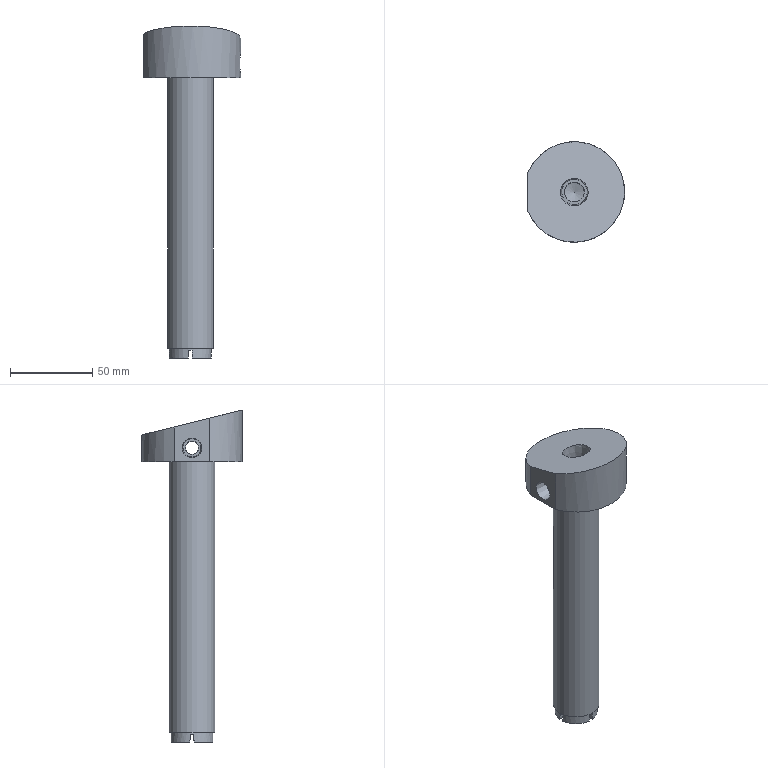Part | STEP file | SLIDE2-INSERT1_id614_x_t | 1 solid | 30 faces | box 59 x 61 x 201.385 mm | volume 145141 mm3 | plane 20 | cylinder 6 | cone 4 | commonest cylinder face diameters 8 x2 12 x1 25.45 x1 27.69 x1 61 x1
STEP:
#1=CARTESIAN_POINT('',(-30.,0.,35.016));
#2=VERTEX_POINT('',#1);
#3=VERTEX_LOOP('',#2);
#4=FACE_BOUND('',#3,.T.);
#5=CARTESIAN_POINT('',(-36.,0.,36.782));
#6=VERTEX_POINT('',#5);
#7=CARTESIAN_POINT('',(-30.,0.,36.782));
#8=DIRECTION('',(0.,0.,1.));
#9=DIRECTION('',(-1.,0.,0.));
#10=AXIS2_PLACEMENT_3D('',#7,#8,#9);
#11=CIRCLE('',#10,6.);
#12=EDGE_CURVE('',#6,#6,#11,.T.);
#13=ORIENTED_EDGE('',*,*,#12,.T.);
#14=EDGE_LOOP('',(#13));
#15=FACE_BOUND('',#14,.T.);
#16=CARTESIAN_POINT('',(-30.,0.,36.782));
#17=DIRECTION('',(0.,0.,1.));
#18=DIRECTION('',(1.,0.,0.));
#19=AXIS2_PLACEMENT_3D('',#16,#17,#18);
#20=CONICAL_SURFACE('',#19,6.,73.607);
#21=ADVANCED_FACE('',(#4,#15),#20,.F.);
#22=ORIENTED_EDGE('',*,*,#12,.F.);
#23=EDGE_LOOP('',(#22));
#24=FACE_BOUND('',#23,.T.);
#25=CARTESIAN_POINT('',(-36.,0.,207.5));
#26=VERTEX_POINT('',#25);
#27=CARTESIAN_POINT('',(-36.,-1.093,207.5));
#28=CARTESIAN_POINT('',(-36.,1.093,207.5));
#29=CARTESIAN_POINT('',(-35.671,2.12,207.039));
#30=CARTESIAN_POINT('',(-34.907,3.546,205.608));
#31=CARTESIAN_POINT('',(-34.475,3.997,204.596));
#32=CARTESIAN_POINT('',(-34.469,4.003,202.427));
#33=CARTESIAN_POINT('',(-34.898,3.559,201.41));
#34=CARTESIAN_POINT('',(-35.668,2.129,199.964));
#35=CARTESIAN_POINT('',(-35.998,1.105,199.503));
#36=CARTESIAN_POINT('',(-36.002,-1.084,199.497));
#37=CARTESIAN_POINT('',(-35.673,-2.115,199.957));
#38=CARTESIAN_POINT('',(-34.908,-3.545,201.389));
#39=CARTESIAN_POINT('',(-34.475,-3.997,202.402));
#40=CARTESIAN_POINT('',(-34.469,-4.003,204.575));
#41=CARTESIAN_POINT('',(-34.9,-3.558,205.593));
#42=CARTESIAN_POINT('',(-35.67,-2.123,207.04));
#43=CARTESIAN_POINT('',(-36.,-1.093,207.5));
#44=CARTESIAN_POINT('',(-36.,1.093,207.5));
#45=B_SPLINE_CURVE_WITH_KNOTS('',3,(#27,#28,#29,#30,#31,#32,#33,#34,#35,#36,#37,#38,#39,#40,#41,#42,#43,#44),.UNSPECIFIED.,.T.,.F.,(2,2,2,2,2,2,2,2,2,2,2),(-0.125,0.,0.125,0.25,0.375,0.5,0.625,0.75,0.875,1.,1.125),.UNSPECIFIED.);
#46=EDGE_CURVE('',#26,#26,#45,.T.);
#47=ORIENTED_EDGE('',*,*,#46,.T.);
#48=EDGE_LOOP('',(#47));
#49=FACE_BOUND('',#48,.T.);
#50=CARTESIAN_POINT('',(-36.,0.,208.));
#51=VERTEX_POINT('',#50);
#52=CARTESIAN_POINT('',(-30.,0.,208.));
#53=DIRECTION('',(0.,0.,1.));
#54=DIRECTION('',(-1.,0.,0.));
#55=AXIS2_PLACEMENT_3D('',#52,#53,#54);
#56=CIRCLE('',#55,6.);
#57=EDGE_CURVE('',#51,#51,#56,.T.);
#58=ORIENTED_EDGE('',*,*,#57,.T.);
#59=EDGE_LOOP('',(#58));
#60=FACE_BOUND('',#59,.T.);
#61=CARTESIAN_POINT('',(-24.,0.,199.5));
#62=VERTEX_POINT('',#61);
#63=CARTESIAN_POINT('',(-24.,-1.093,199.5));
#64=CARTESIAN_POINT('',(-24.,1.093,199.5));
#65=CARTESIAN_POINT('',(-24.329,2.12,199.961));
#66=CARTESIAN_POINT('',(-25.093,3.546,201.392));
#67=CARTESIAN_POINT('',(-25.525,3.997,202.404));
#68=CARTESIAN_POINT('',(-25.531,4.003,204.573));
#69=CARTESIAN_POINT('',(-25.102,3.559,205.59));
#70=CARTESIAN_POINT('',(-24.332,2.129,207.036));
#71=CARTESIAN_POINT('',(-24.002,1.105,207.497));
#72=CARTESIAN_POINT('',(-23.998,-1.084,207.503));
#73=CARTESIAN_POINT('',(-24.327,-2.115,207.043));
#74=CARTESIAN_POINT('',(-25.092,-3.545,205.611));
#75=CARTESIAN_POINT('',(-25.525,-3.997,204.598));
#76=CARTESIAN_POINT('',(-25.531,-4.003,202.425));
#77=CARTESIAN_POINT('',(-25.1,-3.558,201.407));
#78=CARTESIAN_POINT('',(-24.33,-2.123,199.96));
#79=CARTESIAN_POINT('',(-24.,-1.093,199.5));
#80=CARTESIAN_POINT('',(-24.,1.093,199.5));
#81=B_SPLINE_CURVE_WITH_KNOTS('',3,(#63,#64,#65,#66,#67,#68,#69,#70,#71,#72,#73,#74,#75,#76,#77,#78,#79,#80),.UNSPECIFIED.,.T.,.F.,(2,2,2,2,2,2,2,2,2,2,2),(-0.125,0.,0.125,0.25,0.375,0.5,0.625,0.75,0.875,1.,1.125),.UNSPECIFIED.);
#82=EDGE_CURVE('',#62,#62,#81,.T.);
#83=ORIENTED_EDGE('',*,*,#82,.T.);
#84=EDGE_LOOP('',(#83));
#85=FACE_BOUND('',#84,.T.);
#86=CARTESIAN_POINT('',(-30.,0.,236.022));
#87=DIRECTION('',(0.,0.,-1.));
#88=DIRECTION('',(-1.,0.,0.));
#89=AXIS2_PLACEMENT_3D('',#86,#87,#88);
#90=CYLINDRICAL_SURFACE('',#89,6.);
#91=ADVANCED_FACE('',(#24,#49,#60,#85),#90,.F.);
#92=CARTESIAN_POINT('',(-49.5,0.,207.5));
#93=VERTEX_POINT('',#92);
#94=CARTESIAN_POINT('',(-49.5,0.,203.5));
#95=DIRECTION('',(1.,0.,0.));
#96=DIRECTION('',(0.,0.,1.));
#97=AXIS2_PLACEMENT_3D('',#94,#95,#96);
#98=CIRCLE('',#97,4.);
#99=EDGE_CURVE('',#93,#93,#98,.T.);
#100=ORIENTED_EDGE('',*,*,#99,.F.);
#101=EDGE_LOOP('',(#100));
#102=FACE_BOUND('',#101,.T.);
#103=ORIENTED_EDGE('',*,*,#46,.F.);
#104=EDGE_LOOP('',(#103));
#105=FACE_BOUND('',#104,.T.);
#106=CARTESIAN_POINT('',(79.,0.,203.5));
#107=DIRECTION('',(-1.,0.,0.));
#108=DIRECTION('',(0.,0.,1.));
#109=AXIS2_PLACEMENT_3D('',#106,#107,#108);
#110=CYLINDRICAL_SURFACE('',#109,4.);
#111=ADVANCED_FACE('',(#102,#105),#110,.F.);
#112=ORIENTED_EDGE('',*,*,#57,.F.);
#113=EDGE_LOOP('',(#112));
#114=FACE_BOUND('',#113,.T.);
#115=CARTESIAN_POINT('',(-30.,-7.741,208.));
#116=VERTEX_POINT('',#115);
#117=CARTESIAN_POINT('',(-30.,0.,208.));
#118=DIRECTION('',(0.,0.,1.));
#119=DIRECTION('',(0.,-1.,0.));
#120=AXIS2_PLACEMENT_3D('',#117,#118,#119);
#121=CIRCLE('',#120,7.741);
#122=EDGE_CURVE('',#116,#116,#121,.T.);
#123=ORIENTED_EDGE('',*,*,#122,.T.);
#124=EDGE_LOOP('',(#123));
#125=FACE_BOUND('',#124,.T.);
#126=CARTESIAN_POINT('',(-30.,0.,208.));
#127=DIRECTION('',(0.,0.,-1.));
#128=DIRECTION('',(-1.,0.,0.));
#129=AXIS2_PLACEMENT_3D('',#126,#127,#128);
#130=PLANE('',#129);
#131=ADVANCED_FACE('',(#114,#125),#130,.F.);
#132=CARTESIAN_POINT('',(-10.5,0.,207.5));
#133=VERTEX_POINT('',#132);
#134=CARTESIAN_POINT('',(-10.5,0.,203.5));
#135=DIRECTION('',(1.,0.,0.));
#136=DIRECTION('',(0.,0.,1.));
#137=AXIS2_PLACEMENT_3D('',#134,#135,#136);
#138=CIRCLE('',#137,4.);
#139=EDGE_CURVE('',#133,#133,#138,.T.);
#140=ORIENTED_EDGE('',*,*,#139,.T.);
#141=EDGE_LOOP('',(#140));
#142=FACE_BOUND('',#141,.T.);
#143=ORIENTED_EDGE('',*,*,#82,.F.);
#144=EDGE_LOOP('',(#143));
#145=FACE_BOUND('',#144,.T.);
#146=CARTESIAN_POINT('',(79.,0.,203.5));
#147=DIRECTION('',(-1.,0.,0.));
#148=DIRECTION('',(0.,0.,1.));
#149=AXIS2_PLACEMENT_3D('',#146,#147,#148);
#150=CYLINDRICAL_SURFACE('',#149,4.);
#151=ADVANCED_FACE('',(#142,#145),#150,.F.);
#152=ORIENTED_EDGE('',*,*,#99,.T.);
#153=EDGE_LOOP('',(#152));
#154=FACE_BOUND('',#153,.T.);
#155=CARTESIAN_POINT('',(-49.5,0.,209.));
#156=VERTEX_POINT('',#155);
#157=CARTESIAN_POINT('',(-49.5,0.,203.5));
#158=DIRECTION('',(-1.,0.,0.));
#159=DIRECTION('',(0.,0.,1.));
#160=AXIS2_PLACEMENT_3D('',#157,#158,#159);
#161=CIRCLE('',#160,5.5);
#162=EDGE_CURVE('',#156,#156,#161,.T.);
#163=ORIENTED_EDGE('',*,*,#162,.T.);
#164=EDGE_LOOP('',(#163));
#165=FACE_BOUND('',#164,.T.);
#166=CARTESIAN_POINT('',(-49.5,0.,203.5));
#167=DIRECTION('',(-1.,0.,0.));
#168=DIRECTION('',(0.,0.,1.));
#169=AXIS2_PLACEMENT_3D('',#166,#167,#168);
#170=PLANE('',#169);
#171=ADVANCED_FACE('',(#154,#165),#170,.T.);
#172=ORIENTED_EDGE('',*,*,#122,.F.);
#173=EDGE_LOOP('',(#172));
#174=FACE_BOUND('',#173,.T.);
#175=CARTESIAN_POINT('',(-30.,-8.535,220.974));
#176=VERTEX_POINT('',#175);
#177=CARTESIAN_POINT('',(-30.,-0.1282,218.878));
#178=DIRECTION('',(0.,0.2419,0.9703));
#179=DIRECTION('',(0.,-0.9703,0.2419));
#180=AXIS2_PLACEMENT_3D('',#177,#178,#179);
#181=ELLIPSE('',#180,8.664,8.406);
#182=EDGE_CURVE('',#176,#176,#181,.T.);
#183=ORIENTED_EDGE('',*,*,#182,.T.);
#184=EDGE_LOOP('',(#183));
#185=FACE_BOUND('',#184,.T.);
#186=CARTESIAN_POINT('',(-30.,0.,218.911));
#187=DIRECTION('',(0.,0.,1.));
#188=DIRECTION('',(0.,-1.,0.));
#189=AXIS2_PLACEMENT_3D('',#186,#187,#188);
#190=CONICAL_SURFACE('',#189,8.409,3.5);
#191=ADVANCED_FACE('',(#174,#185),#190,.F.);
#192=ORIENTED_EDGE('',*,*,#139,.F.);
#193=EDGE_LOOP('',(#192));
#194=FACE_BOUND('',#193,.T.);
#195=CARTESIAN_POINT('',(-10.5,0.,198.));
#196=VERTEX_POINT('',#195);
#197=CARTESIAN_POINT('',(-10.5,0.,203.5));
#198=DIRECTION('',(1.,0.,0.));
#199=DIRECTION('',(0.,0.,-1.));
#200=AXIS2_PLACEMENT_3D('',#197,#198,#199);
#201=CIRCLE('',#200,5.5);
#202=EDGE_CURVE('',#196,#196,#201,.T.);
#203=ORIENTED_EDGE('',*,*,#202,.T.);
#204=EDGE_LOOP('',(#203));
#205=FACE_BOUND('',#204,.T.);
#206=CARTESIAN_POINT('',(-10.5,0.,203.5));
#207=DIRECTION('',(-1.,0.,0.));
#208=DIRECTION('',(0.,0.,1.));
#209=AXIS2_PLACEMENT_3D('',#206,#207,#208);
#210=PLANE('',#209);
#211=ADVANCED_FACE('',(#194,#205),#210,.F.);
#212=CARTESIAN_POINT('',(-42.661,1.272,25.066));
#213=VERTEX_POINT('',#212);
#214=CARTESIAN_POINT('',(-42.683,1.027,29.749));
#215=VERTEX_POINT('',#214);
#216=CARTESIAN_POINT('',(-30.,0.,49.347));
#217=DIRECTION('',(0.,0.9986,0.05234));
#218=DIRECTION('',(0.,-0.05234,0.9986));
#219=AXIS2_PLACEMENT_3D('',#216,#217,#218);
#220=ELLIPSE('',#219,243.141,12.725);
#221=EDGE_CURVE('',#213,#215,#220,.T.);
#222=ORIENTED_EDGE('',*,*,#221,.F.);
#223=CARTESIAN_POINT('',(-31.273,1.272,25.066));
#224=VERTEX_POINT('',#223);
#225=CARTESIAN_POINT('',(-30.814,1.272,25.066));
#226=DIRECTION('',(1.,0.,0.));
#227=VECTOR('',#226,1.);
#228=LINE('',#225,#227);
#229=EDGE_CURVE('',#213,#224,#228,.T.);
#230=ORIENTED_EDGE('',*,*,#229,.T.);
#231=CARTESIAN_POINT('',(-31.027,1.027,29.749));
#232=VERTEX_POINT('',#231);
#233=CARTESIAN_POINT('',(-31.027,1.027,29.749));
#234=DIRECTION('',(-0.05226,0.05226,-0.9973));
#235=VECTOR('',#234,1.);
#236=LINE('',#233,#235);
#237=EDGE_CURVE('',#232,#224,#236,.T.);
#238=ORIENTED_EDGE('',*,*,#237,.F.);
#239=CARTESIAN_POINT('',(-30.,1.027,29.749));
#240=DIRECTION('',(1.,0.,0.));
#241=VECTOR('',#240,1.);
#242=LINE('',#239,#241);
#243=EDGE_CURVE('',#215,#232,#242,.T.);
#244=ORIENTED_EDGE('',*,*,#243,.F.);
#245=EDGE_LOOP('',(#222,#230,#238,#244));
#246=FACE_OUTER_BOUND('',#245,.T.);
#247=CARTESIAN_POINT('',(-29.406,1.272,25.066));
#248=DIRECTION('',(0.,-0.9986,-0.05234));
#249=DIRECTION('',(0.,0.05234,-0.9986));
#250=AXIS2_PLACEMENT_3D('',#247,#248,#249);
#251=PLANE('',#250);
#252=ADVANCED_FACE('',(#246),#251,.T.);
#253=CARTESIAN_POINT('',(-31.027,-1.027,29.749));
#254=VERTEX_POINT('',#253);
#255=CARTESIAN_POINT('',(-42.683,-1.027,29.749));
#256=VERTEX_POINT('',#255);
#257=CARTESIAN_POINT('',(-30.,-1.027,29.749));
#258=DIRECTION('',(-1.,0.,0.));
#259=VECTOR('',#258,1.);
#260=LINE('',#257,#259);
#261=EDGE_CURVE('',#254,#256,#260,.T.);
#262=ORIENTED_EDGE('',*,*,#261,.F.);
#263=CARTESIAN_POINT('',(-31.273,-1.272,25.066));
#264=VERTEX_POINT('',#263);
#265=CARTESIAN_POINT('',(-31.027,-1.027,29.749));
#266=DIRECTION('',(-0.05226,-0.05226,-0.9973));
#267=VECTOR('',#266,1.);
#268=LINE('',#265,#267);
#269=EDGE_CURVE('',#254,#264,#268,.T.);
#270=ORIENTED_EDGE('',*,*,#269,.T.);
#271=CARTESIAN_POINT('',(-42.661,-1.272,25.066));
#272=VERTEX_POINT('',#271);
#273=CARTESIAN_POINT('',(-30.814,-1.272,25.066));
#274=DIRECTION('',(-1.,0.,0.));
#275=VECTOR('',#274,1.);
#276=LINE('',#273,#275);
#277=EDGE_CURVE('',#264,#272,#276,.T.);
#278=ORIENTED_EDGE('',*,*,#277,.T.);
#279=CARTESIAN_POINT('',(-30.,0.,49.347));
#280=DIRECTION('',(0.,-0.9986,0.05234));
#281=DIRECTION('',(0.,0.05234,0.9986));
#282=AXIS2_PLACEMENT_3D('',#279,#280,#281);
#283=ELLIPSE('',#282,243.141,12.725);
#284=EDGE_CURVE('',#256,#272,#283,.T.);
#285=ORIENTED_EDGE('',*,*,#284,.F.);
#286=EDGE_LOOP('',(#262,#270,#278,#285));
#287=FACE_OUTER_BOUND('',#286,.T.);
#288=CARTESIAN_POINT('',(-29.406,-1.272,25.066));
#289=DIRECTION('',(0.,-0.9986,0.05234));
#290=DIRECTION('',(0.,-0.05234,-0.9986));
#291=AXIS2_PLACEMENT_3D('',#288,#289,#290);
#292=PLANE('',#291);
#293=ADVANCED_FACE('',(#287),#292,.F.);
#294=CARTESIAN_POINT('',(-31.273,-12.661,25.066));
#295=VERTEX_POINT('',#294);
#296=CARTESIAN_POINT('',(-30.,0.,25.066));
#297=DIRECTION('',(0.,0.,1.));
#298=DIRECTION('',(1.,0.,0.));
#299=AXIS2_PLACEMENT_3D('',#296,#297,#298);
#300=CIRCLE('',#299,12.725);
#301=EDGE_CURVE('',#272,#295,#300,.T.);
#302=ORIENTED_EDGE('',*,*,#301,.F.);
#303=ORIENTED_EDGE('',*,*,#277,.F.);
#304=CARTESIAN_POINT('',(-31.273,-14.792,25.066));
#305=DIRECTION('',(0.,-1.,0.));
#306=VECTOR('',#305,1.);
#307=LINE('',#304,#306);
#308=EDGE_CURVE('',#264,#295,#307,.T.);
#309=ORIENTED_EDGE('',*,*,#308,.T.);
#310=EDGE_LOOP('',(#302,#303,#309));
#311=FACE_OUTER_BOUND('',#310,.T.);
#312=CARTESIAN_POINT('',(-30.814,0.,25.066));
#313=DIRECTION('',(0.,0.,1.));
#314=DIRECTION('',(1.,0.,0.));
#315=AXIS2_PLACEMENT_3D('',#312,#313,#314);
#316=PLANE('',#315);
#317=ADVANCED_FACE('',(#311),#316,.F.);
#318=CARTESIAN_POINT('',(-31.027,-12.683,29.749));
#319=VERTEX_POINT('',#318);
#320=CARTESIAN_POINT('',(-31.027,0.,29.749));
#321=DIRECTION('',(0.,1.,0.));
#322=VECTOR('',#321,1.);
#323=LINE('',#320,#322);
#324=EDGE_CURVE('',#319,#254,#323,.T.);
#325=ORIENTED_EDGE('',*,*,#324,.F.);
#326=CARTESIAN_POINT('',(-30.,0.,49.347));
#327=DIRECTION('',(-0.9986,0.,0.05234));
#328=DIRECTION('',(0.05234,0.,0.9986));
#329=AXIS2_PLACEMENT_3D('',#326,#327,#328);
#330=ELLIPSE('',#329,243.141,12.725);
#331=EDGE_CURVE('',#295,#319,#330,.T.);
#332=ORIENTED_EDGE('',*,*,#331,.F.);
#333=ORIENTED_EDGE('',*,*,#308,.F.);
#334=ORIENTED_EDGE('',*,*,#269,.F.);
#335=EDGE_LOOP('',(#325,#332,#333,#334));
#336=FACE_OUTER_BOUND('',#335,.T.);
#337=CARTESIAN_POINT('',(-31.273,-14.792,25.066));
#338=DIRECTION('',(-0.9986,0.,0.05234));
#339=DIRECTION('',(0.05234,0.,0.9986));
#340=AXIS2_PLACEMENT_3D('',#337,#338,#339);
#341=PLANE('',#340);
#342=ADVANCED_FACE('',(#336),#341,.F.);
#343=ORIENTED_EDGE('',*,*,#237,.T.);
#344=CARTESIAN_POINT('',(-31.273,12.661,25.066));
#345=VERTEX_POINT('',#344);
#346=CARTESIAN_POINT('',(-31.273,0.,25.066));
#347=DIRECTION('',(0.,1.,0.));
#348=VECTOR('',#347,1.);
#349=LINE('',#346,#348);
#350=EDGE_CURVE('',#224,#345,#349,.T.);
#351=ORIENTED_EDGE('',*,*,#350,.T.);
#352=CARTESIAN_POINT('',(-31.027,12.683,29.749));
#353=VERTEX_POINT('',#352);
#354=CARTESIAN_POINT('',(-30.,0.,49.347));
#355=DIRECTION('',(-0.9986,0.,0.05234));
#356=DIRECTION('',(0.05234,0.,0.9986));
#357=AXIS2_PLACEMENT_3D('',#354,#355,#356);
#358=ELLIPSE('',#357,243.141,12.725);
#359=EDGE_CURVE('',#353,#345,#358,.T.);
#360=ORIENTED_EDGE('',*,*,#359,.F.);
#361=CARTESIAN_POINT('',(-31.027,0.,29.749));
#362=DIRECTION('',(0.,1.,0.));
#363=VECTOR('',#362,1.);
#364=LINE('',#361,#363);
#365=EDGE_CURVE('',#232,#353,#364,.T.);
#366=ORIENTED_EDGE('',*,*,#365,.F.);
#367=EDGE_LOOP('',(#343,#351,#360,#366));
#368=FACE_OUTER_BOUND('',#367,.T.);
#369=CARTESIAN_POINT('',(-31.273,14.792,25.066));
#370=DIRECTION('',(0.9986,0.,-0.05234));
#371=DIRECTION('',(-0.05234,0.,-0.9986));
#372=AXIS2_PLACEMENT_3D('',#369,#370,#371);
#373=PLANE('',#372);
#374=ADVANCED_FACE('',(#368),#373,.T.);
#375=CARTESIAN_POINT('',(-30.,0.,25.066));
#376=DIRECTION('',(0.,0.,1.));
#377=DIRECTION('',(1.,0.,0.));
#378=AXIS2_PLACEMENT_3D('',#375,#376,#377);
#379=CIRCLE('',#378,12.725);
#380=EDGE_CURVE('',#345,#213,#379,.T.);
#381=ORIENTED_EDGE('',*,*,#380,.F.);
#382=ORIENTED_EDGE('',*,*,#350,.F.);
#383=ORIENTED_EDGE('',*,*,#229,.F.);
#384=EDGE_LOOP('',(#381,#382,#383));
#385=FACE_OUTER_BOUND('',#384,.T.);
#386=CARTESIAN_POINT('',(-30.814,0.,25.066));
#387=DIRECTION('',(0.,0.,1.));
#388=DIRECTION('',(1.,0.,0.));
#389=AXIS2_PLACEMENT_3D('',#386,#387,#388);
#390=PLANE('',#389);
#391=ADVANCED_FACE('',(#385),#390,.F.);
#392=CARTESIAN_POINT('',(-17.317,-1.027,29.749));
#393=VERTEX_POINT('',#392);
#394=CARTESIAN_POINT('',(-28.973,-1.027,29.749));
#395=VERTEX_POINT('',#394);
#396=CARTESIAN_POINT('',(-30.,-1.027,29.749));
#397=DIRECTION('',(-1.,0.,0.));
#398=VECTOR('',#397,1.);
#399=LINE('',#396,#398);
#400=EDGE_CURVE('',#393,#395,#399,.T.);
#401=ORIENTED_EDGE('',*,*,#400,.F.);
#402=CARTESIAN_POINT('',(-17.339,-1.272,25.066));
#403=VERTEX_POINT('',#402);
#404=CARTESIAN_POINT('',(-30.,0.,49.347));
#405=DIRECTION('',(0.,-0.9986,0.05234));
#406=DIRECTION('',(0.,0.05234,0.9986));
#407=AXIS2_PLACEMENT_3D('',#404,#405,#406);
#408=ELLIPSE('',#407,243.141,12.725);
#409=EDGE_CURVE('',#403,#393,#408,.T.);
#410=ORIENTED_EDGE('',*,*,#409,.F.);
#411=CARTESIAN_POINT('',(-28.727,-1.272,25.066));
#412=VERTEX_POINT('',#411);
#413=CARTESIAN_POINT('',(-30.814,-1.272,25.066));
#414=DIRECTION('',(-1.,0.,0.));
#415=VECTOR('',#414,1.);
#416=LINE('',#413,#415);
#417=EDGE_CURVE('',#403,#412,#416,.T.);
#418=ORIENTED_EDGE('',*,*,#417,.T.);
#419=CARTESIAN_POINT('',(-28.727,-1.272,25.066));
#420=DIRECTION('',(-0.05226,0.05226,0.9973));
#421=VECTOR('',#420,1.);
#422=LINE('',#419,#421);
#423=EDGE_CURVE('',#412,#395,#422,.T.);
#424=ORIENTED_EDGE('',*,*,#423,.T.);
#425=EDGE_LOOP('',(#401,#410,#418,#424));
#426=FACE_OUTER_BOUND('',#425,.T.);
#427=CARTESIAN_POINT('',(-15.409,-1.272,25.066));
#428=DIRECTION('',(0.,-0.9986,0.05234));
#429=DIRECTION('',(0.,-0.05234,-0.9986));
#430=AXIS2_PLACEMENT_3D('',#427,#428,#429);
#431=PLANE('',#430);
#432=ADVANCED_FACE('',(#426),#431,.F.);
#433=CARTESIAN_POINT('',(-28.973,-12.683,29.749));
#434=VERTEX_POINT('',#433);
#435=CARTESIAN_POINT('',(-30.,0.,29.749));
#436=DIRECTION('',(0.,0.,1.));
#437=DIRECTION('',(1.,0.,0.));
#438=AXIS2_PLACEMENT_3D('',#435,#436,#437);
#439=CIRCLE('',#438,12.725);
#440=EDGE_CURVE('',#319,#434,#439,.T.);
#441=ORIENTED_EDGE('',*,*,#440,.F.);
#442=ORIENTED_EDGE('',*,*,#324,.T.);
#443=ORIENTED_EDGE('',*,*,#261,.T.);
#444=CARTESIAN_POINT('',(-30.,0.,29.749));
#445=DIRECTION('',(0.,0.,1.));
#446=DIRECTION('',(1.,0.,0.));
#447=AXIS2_PLACEMENT_3D('',#444,#445,#446);
#448=CIRCLE('',#447,12.725);
#449=EDGE_CURVE('',#215,#256,#448,.T.);
#450=ORIENTED_EDGE('',*,*,#449,.F.);
#451=ORIENTED_EDGE('',*,*,#243,.T.);
#452=ORIENTED_EDGE('',*,*,#365,.T.);
#453=CARTESIAN_POINT('',(-28.973,12.683,29.749));
#454=VERTEX_POINT('',#453);
#455=CARTESIAN_POINT('',(-30.,0.,29.749));
#456=DIRECTION('',(0.,0.,1.));
#457=DIRECTION('',(1.,0.,0.));
#458=AXIS2_PLACEMENT_3D('',#455,#456,#457);
#459=CIRCLE('',#458,12.725);
#460=EDGE_CURVE('',#454,#353,#459,.T.);
#461=ORIENTED_EDGE('',*,*,#460,.F.);
#462=CARTESIAN_POINT('',(-28.973,1.027,29.749));
#463=VERTEX_POINT('',#462);
#464=CARTESIAN_POINT('',(-28.973,-0.5939,29.749));
#465=DIRECTION('',(0.,1.,0.));
#466=VECTOR('',#465,1.);
#467=LINE('',#464,#466);
#468=EDGE_CURVE('',#463,#454,#467,.T.);
#469=ORIENTED_EDGE('',*,*,#468,.F.);
#470=CARTESIAN_POINT('',(-17.317,1.027,29.749));
#471=VERTEX_POINT('',#470);
#472=CARTESIAN_POINT('',(-15.409,1.027,29.749));
#473=DIRECTION('',(-1.,0.,0.));
#474=VECTOR('',#473,1.);
#475=LINE('',#472,#474);
#476=EDGE_CURVE('',#471,#463,#475,.T.);
#477=ORIENTED_EDGE('',*,*,#476,.F.);
#478=CARTESIAN_POINT('',(-30.,0.,29.749));
#479=DIRECTION('',(0.,0.,1.));
#480=DIRECTION('',(1.,0.,0.));
#481=AXIS2_PLACEMENT_3D('',#478,#479,#480);
#482=CIRCLE('',#481,12.725);
#483=EDGE_CURVE('',#393,#471,#482,.T.);
#484=ORIENTED_EDGE('',*,*,#483,.F.);
#485=ORIENTED_EDGE('',*,*,#400,.T.);
#486=CARTESIAN_POINT('',(-28.973,0.5939,29.749));
#487=DIRECTION('',(0.,-1.,0.));
#488=VECTOR('',#487,1.);
#489=LINE('',#486,#488);
#490=EDGE_CURVE('',#395,#434,#489,.T.);
#491=ORIENTED_EDGE('',*,*,#490,.T.);
#492=EDGE_LOOP('',(#441,#442,#443,#450,#451,#452,#461,#469,#477,#484,#485,#491));
#493=FACE_OUTER_BOUND('',#492,.T.);
#494=CARTESIAN_POINT('',(-30.,0.,29.749));
#495=DIRECTION('',(0.,0.,-1.));
#496=DIRECTION('',(-1.,0.,0.));
#497=AXIS2_PLACEMENT_3D('',#494,#495,#496);
#498=PLANE('',#497);
#499=ADVANCED_FACE('',(#493),#498,.T.);
#500=CARTESIAN_POINT('',(-28.727,1.272,25.066));
#501=VERTEX_POINT('',#500);
#502=CARTESIAN_POINT('',(-28.727,1.272,25.066));
#503=DIRECTION('',(-0.05226,-0.05226,0.9973));
#504=VECTOR('',#503,1.);
#505=LINE('',#502,#504);
#506=EDGE_CURVE('',#501,#463,#505,.T.);
#507=ORIENTED_EDGE('',*,*,#506,.F.);
#508=CARTESIAN_POINT('',(-17.339,1.272,25.066));
#509=VERTEX_POINT('',#508);
#510=CARTESIAN_POINT('',(-30.814,1.272,25.066));
#511=DIRECTION('',(1.,0.,0.));
#512=VECTOR('',#511,1.);
#513=LINE('',#510,#512);
#514=EDGE_CURVE('',#501,#509,#513,.T.);
#515=ORIENTED_EDGE('',*,*,#514,.T.);
#516=CARTESIAN_POINT('',(-30.,0.,49.347));
#517=DIRECTION('',(0.,0.9986,0.05234));
#518=DIRECTION('',(0.,-0.05234,0.9986));
#519=AXIS2_PLACEMENT_3D('',#516,#517,#518);
#520=ELLIPSE('',#519,243.141,12.725);
#521=EDGE_CURVE('',#471,#509,#520,.T.);
#522=ORIENTED_EDGE('',*,*,#521,.F.);
#523=ORIENTED_EDGE('',*,*,#476,.T.);
#524=EDGE_LOOP('',(#507,#515,#522,#523));
#525=FACE_OUTER_BOUND('',#524,.T.);
#526=CARTESIAN_POINT('',(-15.409,1.272,25.066));
#527=DIRECTION('',(0.,-0.9986,-0.05234));
#528=DIRECTION('',(0.,0.05234,-0.9986));
#529=AXIS2_PLACEMENT_3D('',#526,#527,#528);
#530=PLANE('',#529);
#531=ADVANCED_FACE('',(#525),#530,.T.);
#532=CARTESIAN_POINT('',(-28.727,12.661,25.066));
#533=VERTEX_POINT('',#532);
#534=CARTESIAN_POINT('',(-28.727,-0.5939,25.066));
#535=DIRECTION('',(0.,-1.,0.));
#536=VECTOR('',#535,1.);
#537=LINE('',#534,#536);
#538=EDGE_CURVE('',#533,#501,#537,.T.);
#539=ORIENTED_EDGE('',*,*,#538,.F.);
#540=CARTESIAN_POINT('',(-30.,0.,25.066));
#541=DIRECTION('',(0.,0.,1.));
#542=DIRECTION('',(1.,0.,0.));
#543=AXIS2_PLACEMENT_3D('',#540,#541,#542);
#544=CIRCLE('',#543,12.725);
#545=EDGE_CURVE('',#509,#533,#544,.T.);
#546=ORIENTED_EDGE('',*,*,#545,.F.);
#547=ORIENTED_EDGE('',*,*,#514,.F.);
#548=EDGE_LOOP('',(#539,#546,#547));
#549=FACE_OUTER_BOUND('',#548,.T.);
#550=CARTESIAN_POINT('',(-30.814,0.,25.066));
#551=DIRECTION('',(0.,0.,1.));
#552=DIRECTION('',(1.,0.,0.));
#553=AXIS2_PLACEMENT_3D('',#550,#551,#552);
#554=PLANE('',#553);
#555=ADVANCED_FACE('',(#549),#554,.F.);
#556=CARTESIAN_POINT('',(-30.,0.,49.347));
#557=DIRECTION('',(0.9986,0.,0.05234));
#558=DIRECTION('',(-0.05234,0.,0.9986));
#559=AXIS2_PLACEMENT_3D('',#556,#557,#558);
#560=ELLIPSE('',#559,243.141,12.725);
#561=EDGE_CURVE('',#533,#454,#560,.T.);
#562=ORIENTED_EDGE('',*,*,#561,.F.);
#563=ORIENTED_EDGE('',*,*,#538,.T.);
#564=ORIENTED_EDGE('',*,*,#506,.T.);
#565=ORIENTED_EDGE('',*,*,#468,.T.);
#566=EDGE_LOOP('',(#562,#563,#564,#565));
#567=FACE_OUTER_BOUND('',#566,.T.);
#568=CARTESIAN_POINT('',(-28.727,-0.5939,25.066));
#569=DIRECTION('',(-0.9986,0.,-0.05234));
#570=DIRECTION('',(-0.05234,0.,0.9986));
#571=AXIS2_PLACEMENT_3D('',#568,#569,#570);
#572=PLANE('',#571);
#573=ADVANCED_FACE('',(#567),#572,.T.);
#574=ORIENTED_EDGE('',*,*,#490,.F.);
#575=ORIENTED_EDGE('',*,*,#423,.F.);
#576=CARTESIAN_POINT('',(-28.727,-12.661,25.066));
#577=VERTEX_POINT('',#576);
#578=CARTESIAN_POINT('',(-28.727,0.,25.066));
#579=DIRECTION('',(0.,-1.,0.));
#580=VECTOR('',#579,1.);
#581=LINE('',#578,#580);
#582=EDGE_CURVE('',#412,#577,#581,.T.);
#583=ORIENTED_EDGE('',*,*,#582,.T.);
#584=CARTESIAN_POINT('',(-30.,0.,49.347));
#585=DIRECTION('',(0.9986,0.,0.05234));
#586=DIRECTION('',(-0.05234,0.,0.9986));
#587=AXIS2_PLACEMENT_3D('',#584,#585,#586);
#588=ELLIPSE('',#587,243.141,12.725);
#589=EDGE_CURVE('',#434,#577,#588,.T.);
#590=ORIENTED_EDGE('',*,*,#589,.F.);
#591=EDGE_LOOP('',(#574,#575,#583,#590));
#592=FACE_OUTER_BOUND('',#591,.T.);
#593=CARTESIAN_POINT('',(-28.727,0.5939,25.066));
#594=DIRECTION('',(0.9986,0.,0.05234));
#595=DIRECTION('',(0.05234,0.,-0.9986));
#596=AXIS2_PLACEMENT_3D('',#593,#594,#595);
#597=PLANE('',#596);
#598=ADVANCED_FACE('',(#592),#597,.F.);
#599=CARTESIAN_POINT('',(-30.,0.,25.066));
#600=DIRECTION('',(0.,0.,1.));
#601=DIRECTION('',(1.,0.,0.));
#602=AXIS2_PLACEMENT_3D('',#599,#600,#601);
#603=CIRCLE('',#602,12.725);
#604=EDGE_CURVE('',#577,#403,#603,.T.);
#605=ORIENTED_EDGE('',*,*,#604,.F.);
#606=ORIENTED_EDGE('',*,*,#582,.F.);
#607=ORIENTED_EDGE('',*,*,#417,.F.);
#608=EDGE_LOOP('',(#605,#606,#607));
#609=FACE_OUTER_BOUND('',#608,.T.);
#610=CARTESIAN_POINT('',(-30.814,0.,25.066));
#611=DIRECTION('',(0.,0.,1.));
#612=DIRECTION('',(1.,0.,0.));
#613=AXIS2_PLACEMENT_3D('',#610,#611,#612);
#614=PLANE('',#613);
#615=ADVANCED_FACE('',(#609),#614,.F.);
#616=ORIENTED_EDGE('',*,*,#162,.F.);
#617=EDGE_LOOP('',(#616));
#618=FACE_BOUND('',#617,.T.);
#619=CARTESIAN_POINT('',(-58.5,0.,209.409));
#620=VERTEX_POINT('',#619);
#621=CARTESIAN_POINT('',(-58.5,0.,203.5));
#622=DIRECTION('',(-1.,0.,0.));
#623=DIRECTION('',(0.,0.,1.));
#624=AXIS2_PLACEMENT_3D('',#621,#622,#623);
#625=CIRCLE('',#624,5.909);
#626=EDGE_CURVE('',#620,#620,#625,.T.);
#627=ORIENTED_EDGE('',*,*,#626,.T.);
#628=EDGE_LOOP('',(#627));
#629=FACE_BOUND('',#628,.T.);
#630=CARTESIAN_POINT('',(-58.5,0.,203.5));
#631=DIRECTION('',(-1.,0.,0.));
#632=DIRECTION('',(0.,0.,1.));
#633=AXIS2_PLACEMENT_3D('',#630,#631,#632);
#634=CONICAL_SURFACE('',#633,5.909,2.603);
#635=ADVANCED_FACE('',(#618,#629),#634,.F.);
#636=ORIENTED_EDGE('',*,*,#182,.F.);
#637=EDGE_LOOP('',(#636));
#638=FACE_BOUND('',#637,.T.);
#639=CARTESIAN_POINT('',(-58.5,10.863,216.138));
#640=VERTEX_POINT('',#639);
#641=CARTESIAN_POINT('',(-58.5,-10.863,221.554));
#642=VERTEX_POINT('',#641);
#643=CARTESIAN_POINT('',(-58.5,10.863,216.138));
#644=DIRECTION('',(0.,-0.9703,0.2419));
#645=VECTOR('',#644,1.);
#646=LINE('',#643,#645);
#647=EDGE_CURVE('',#640,#642,#646,.T.);
#648=ORIENTED_EDGE('',*,*,#647,.T.);
#649=CARTESIAN_POINT('',(-30.,0.,218.846));
#650=DIRECTION('',(0.,-0.2419,-0.9703));
#651=DIRECTION('',(0.,-0.9703,0.2419));
#652=AXIS2_PLACEMENT_3D('',#649,#650,#651);
#653=ELLIPSE('',#652,31.434,30.5);
#654=EDGE_CURVE('',#640,#642,#653,.T.);
#655=ORIENTED_EDGE('',*,*,#654,.F.);
#656=EDGE_LOOP('',(#648,#655));
#657=FACE_BOUND('',#656,.T.);
#658=CARTESIAN_POINT('',(-90.,-21.1,224.107));
#659=DIRECTION('',(0.,-0.2419,-0.9703));
#660=DIRECTION('',(0.,0.9703,-0.2419));
#661=AXIS2_PLACEMENT_3D('',#658,#659,#660);
#662=PLANE('',#661);
#663=ADVANCED_FACE('',(#638,#657),#662,.F.);
#664=ORIENTED_EDGE('',*,*,#202,.F.);
#665=EDGE_LOOP('',(#664));
#666=FACE_BOUND('',#665,.T.);
#667=CARTESIAN_POINT('',(0.5,-0.000000496,197.5));
#668=VERTEX_POINT('',#667);
#669=CARTESIAN_POINT('',(0.5,1.586,197.5));
#670=CARTESIAN_POINT('',(0.5,-1.586,197.5));
#671=CARTESIAN_POINT('',(0.3591,-3.131,198.157));
#672=CARTESIAN_POINT('',(0.05178,-5.326,200.367));
#673=CARTESIAN_POINT('',(-0.09038,-5.972,201.93));
#674=CARTESIAN_POINT('',(-0.09084,-5.974,205.062));
#675=CARTESIAN_POINT('',(0.04986,-5.339,206.618));
#676=CARTESIAN_POINT('',(0.3604,-3.122,208.853));
#677=CARTESIAN_POINT('',(0.5,-1.586,209.5));
#678=CARTESIAN_POINT('',(0.5,1.586,209.5));
#679=CARTESIAN_POINT('',(0.3591,3.131,208.843));
#680=CARTESIAN_POINT('',(0.05178,5.326,206.633));
#681=CARTESIAN_POINT('',(-0.09038,5.972,205.071));
#682=CARTESIAN_POINT('',(-0.09084,5.974,201.938));
#683=CARTESIAN_POINT('',(0.04987,5.339,200.382));
#684=CARTESIAN_POINT('',(0.3604,3.122,198.147));
#685=CARTESIAN_POINT('',(0.5,1.586,197.5));
#686=CARTESIAN_POINT('',(0.5,-1.586,197.5));
#687=B_SPLINE_CURVE_WITH_KNOTS('',3,(#669,#670,#671,#672,#673,#674,#675,#676,#677,#678,#679,#680,#681,#682,#683,#684,#685,#686),.UNSPECIFIED.,.T.,.F.,(2,2,2,2,2,2,2,2,2,2,2),(-0.125,0.,0.125,0.25,0.375,0.5,0.625,0.75,0.875,1.,1.125),.UNSPECIFIED.);
#688=EDGE_CURVE('',#668,#668,#687,.T.);
#689=ORIENTED_EDGE('',*,*,#688,.F.);
#690=EDGE_LOOP('',(#689));
#691=FACE_BOUND('',#690,.T.);
#692=CARTESIAN_POINT('',(0.566,0.,203.5));
#693=DIRECTION('',(1.,0.,0.));
#694=DIRECTION('',(0.,0.,-1.));
#695=AXIS2_PLACEMENT_3D('',#692,#693,#694);
#696=CONICAL_SURFACE('',#695,6.003,2.603);
#697=ADVANCED_FACE('',(#666,#691),#696,.F.);
#698=CARTESIAN_POINT('',(-17.275,0.,31.072));
#699=VERTEX_POINT('',#698);
#700=CARTESIAN_POINT('',(-30.,0.,31.072));
#701=DIRECTION('',(0.,0.,-1.));
#702=DIRECTION('',(1.,0.,0.));
#703=AXIS2_PLACEMENT_3D('',#700,#701,#702);
#704=CIRCLE('',#703,12.725);
#705=EDGE_CURVE('',#699,#699,#704,.T.);
#706=ORIENTED_EDGE('',*,*,#705,.T.);
#707=EDGE_LOOP('',(#706));
#708=FACE_BOUND('',#707,.T.);
#709=ORIENTED_EDGE('',*,*,#589,.T.);
#710=ORIENTED_EDGE('',*,*,#604,.T.);
#711=ORIENTED_EDGE('',*,*,#409,.T.);
#712=ORIENTED_EDGE('',*,*,#483,.T.);
#713=ORIENTED_EDGE('',*,*,#521,.T.);
#714=ORIENTED_EDGE('',*,*,#545,.T.);
#715=ORIENTED_EDGE('',*,*,#561,.T.);
#716=ORIENTED_EDGE('',*,*,#460,.T.);
#717=ORIENTED_EDGE('',*,*,#359,.T.);
#718=ORIENTED_EDGE('',*,*,#380,.T.);
#719=ORIENTED_EDGE('',*,*,#221,.T.);
#720=ORIENTED_EDGE('',*,*,#449,.T.);
#721=ORIENTED_EDGE('',*,*,#284,.T.);
#722=ORIENTED_EDGE('',*,*,#301,.T.);
#723=ORIENTED_EDGE('',*,*,#331,.T.);
#724=ORIENTED_EDGE('',*,*,#440,.T.);
#725=EDGE_LOOP('',(#709,#710,#711,#712,#713,#714,#715,#716,#717,#718,#719,#720,#721,#722,#723,#724));
#726=FACE_BOUND('',#725,.T.);
#727=CARTESIAN_POINT('',(-30.,0.,27.611));
#728=DIRECTION('',(0.,0.,1.));
#729=DIRECTION('',(1.,0.,0.));
#730=AXIS2_PLACEMENT_3D('',#727,#728,#729);
#731=CYLINDRICAL_SURFACE('',#730,12.725);
#732=ADVANCED_FACE('',(#708,#726),#731,.T.);
#733=ORIENTED_EDGE('',*,*,#626,.F.);
#734=EDGE_LOOP('',(#733));
#735=FACE_BOUND('',#734,.T.);
#736=ORIENTED_EDGE('',*,*,#647,.F.);
#737=CARTESIAN_POINT('',(-58.5,10.863,195.003));
#738=VERTEX_POINT('',#737);
#739=CARTESIAN_POINT('',(-58.5,10.863,195.003));
#740=DIRECTION('',(0.,0.,1.));
#741=VECTOR('',#740,1.);
#742=LINE('',#739,#741);
#743=EDGE_CURVE('',#738,#640,#742,.T.);
#744=ORIENTED_EDGE('',*,*,#743,.F.);
#745=CARTESIAN_POINT('',(-58.5,-10.863,195.003));
#746=VERTEX_POINT('',#745);
#747=CARTESIAN_POINT('',(-58.5,0.,195.003));
#748=DIRECTION('',(0.,-1.,0.));
#749=VECTOR('',#748,1.);
#750=LINE('',#747,#749);
#751=EDGE_CURVE('',#738,#746,#750,.T.);
#752=ORIENTED_EDGE('',*,*,#751,.T.);
#753=CARTESIAN_POINT('',(-58.5,-10.863,195.003));
#754=DIRECTION('',(0.,0.,-1.));
#755=VECTOR('',#754,1.);
#756=LINE('',#753,#755);
#757=EDGE_CURVE('',#642,#746,#756,.T.);
#758=ORIENTED_EDGE('',*,*,#757,.F.);
#759=EDGE_LOOP('',(#736,#744,#752,#758));
#760=FACE_BOUND('',#759,.T.);
#761=CARTESIAN_POINT('',(-58.5,-10.863,217.003));
#762=DIRECTION('',(1.,0.,0.));
#763=DIRECTION('',(0.,0.,-1.));
#764=AXIS2_PLACEMENT_3D('',#761,#762,#763);
#765=PLANE('',#764);
#766=ADVANCED_FACE('',(#735,#760),#765,.F.);
#767=ORIENTED_EDGE('',*,*,#688,.T.);
#768=EDGE_LOOP('',(#767));
#769=FACE_BOUND('',#768,.T.);
#770=ORIENTED_EDGE('',*,*,#757,.T.);
#771=CARTESIAN_POINT('',(-30.,0.,195.003));
#772=DIRECTION('',(0.,0.,1.));
#773=DIRECTION('',(1.,0.,0.));
#774=AXIS2_PLACEMENT_3D('',#771,#772,#773);
#775=CIRCLE('',#774,30.5);
#776=EDGE_CURVE('',#746,#738,#775,.T.);
#777=ORIENTED_EDGE('',*,*,#776,.T.);
#778=ORIENTED_EDGE('',*,*,#743,.T.);
#779=ORIENTED_EDGE('',*,*,#654,.T.);
#780=EDGE_LOOP('',(#770,#777,#778,#779));
#781=FACE_BOUND('',#780,.T.);
#782=CARTESIAN_POINT('',(-30.,0.,195.003));
#783=DIRECTION('',(0.,0.,1.));
#784=DIRECTION('',(1.,0.,0.));
#785=AXIS2_PLACEMENT_3D('',#782,#783,#784);
#786=CYLINDRICAL_SURFACE('',#785,30.5);
#787=ADVANCED_FACE('',(#769,#781),#786,.T.);
#788=ORIENTED_EDGE('',*,*,#705,.F.);
#789=EDGE_LOOP('',(#788));
#790=FACE_BOUND('',#789,.T.);
#791=CARTESIAN_POINT('',(-16.155,0.,31.072));
#792=VERTEX_POINT('',#791);
#793=CARTESIAN_POINT('',(-30.,0.,31.072));
#794=DIRECTION('',(0.,0.,1.));
#795=DIRECTION('',(1.,0.,0.));
#796=AXIS2_PLACEMENT_3D('',#793,#794,#795);
#797=CIRCLE('',#796,13.845);
#798=EDGE_CURVE('',#792,#792,#797,.T.);
#799=ORIENTED_EDGE('',*,*,#798,.F.);
#800=EDGE_LOOP('',(#799));
#801=FACE_BOUND('',#800,.T.);
#802=CARTESIAN_POINT('',(-30.,0.,31.072));
#803=DIRECTION('',(0.,0.,1.));
#804=DIRECTION('',(1.,0.,0.));
#805=AXIS2_PLACEMENT_3D('',#802,#803,#804);
#806=PLANE('',#805);
#807=ADVANCED_FACE('',(#790,#801),#806,.F.);
#808=CARTESIAN_POINT('',(-16.155,0.,195.003));
#809=VERTEX_POINT('',#808);
#810=CARTESIAN_POINT('',(-30.,0.,195.003));
#811=DIRECTION('',(0.,0.,-1.));
#812=DIRECTION('',(1.,0.,0.));
#813=AXIS2_PLACEMENT_3D('',#810,#811,#812);
#814=CIRCLE('',#813,13.845);
#815=EDGE_CURVE('',#809,#809,#814,.T.);
#816=ORIENTED_EDGE('',*,*,#815,.F.);
#817=EDGE_LOOP('',(#816));
#818=FACE_BOUND('',#817,.T.);
#819=ORIENTED_EDGE('',*,*,#751,.F.);
#820=ORIENTED_EDGE('',*,*,#776,.F.);
#821=EDGE_LOOP('',(#819,#820));
#822=FACE_BOUND('',#821,.T.);
#823=CARTESIAN_POINT('',(0.,0.,195.003));
#824=DIRECTION('',(0.,0.,1.));
#825=DIRECTION('',(1.,0.,0.));
#826=AXIS2_PLACEMENT_3D('',#823,#824,#825);
#827=PLANE('',#826);
#828=ADVANCED_FACE('',(#818,#822),#827,.F.);
#829=ORIENTED_EDGE('',*,*,#798,.T.);
#830=EDGE_LOOP('',(#829));
#831=FACE_BOUND('',#830,.T.);
#832=ORIENTED_EDGE('',*,*,#815,.T.);
#833=EDGE_LOOP('',(#832));
#834=FACE_BOUND('',#833,.T.);
#835=CARTESIAN_POINT('',(-30.,0.,195.003));
#836=DIRECTION('',(0.,0.,1.));
#837=DIRECTION('',(1.,0.,0.));
#838=AXIS2_PLACEMENT_3D('',#835,#836,#837);
#839=CYLINDRICAL_SURFACE('',#838,13.845);
#840=ADVANCED_FACE('',(#831,#834),#839,.T.);
#841=CLOSED_SHELL('',(#21,#91,#111,#131,#151,#171,#191,#211,#252,#293,#317,#342,#374,#391,#432,#499,#531,#555,#573,#598,#615,#635,#663,#697,#732,#766,#787,#807,#828,#840));
#842=MANIFOLD_SOLID_BREP('',#841);
#843=(LENGTH_UNIT()NAMED_UNIT(*)SI_UNIT(.MILLI.,.METRE.));
#844=UNCERTAINTY_MEASURE_WITH_UNIT(LENGTH_MEASURE(0.0508),#843,'','');
#845=(NAMED_UNIT(*)PLANE_ANGLE_UNIT()SI_UNIT($,.RADIAN.));
#846=PLANE_ANGLE_MEASURE_WITH_UNIT(PLANE_ANGLE_MEASURE(0.01745),#845);
#847=DIMENSIONAL_EXPONENTS(0.,0.,0.,0.,0.,0.,0.);
#848=(CONVERSION_BASED_UNIT('DEGREE',#846)NAMED_UNIT(#847)PLANE_ANGLE_UNIT());
#849=(NAMED_UNIT(*)SI_UNIT($,.STERADIAN.)SOLID_ANGLE_UNIT());
#850=(GEOMETRIC_REPRESENTATION_CONTEXT(3)GLOBAL_UNCERTAINTY_ASSIGNED_CONTEXT((#844))GLOBAL_UNIT_ASSIGNED_CONTEXT((#843,#848,#849))REPRESENTATION_CONTEXT('',''));
#851=ADVANCED_BREP_SHAPE_REPRESENTATION('',(#842),#850);